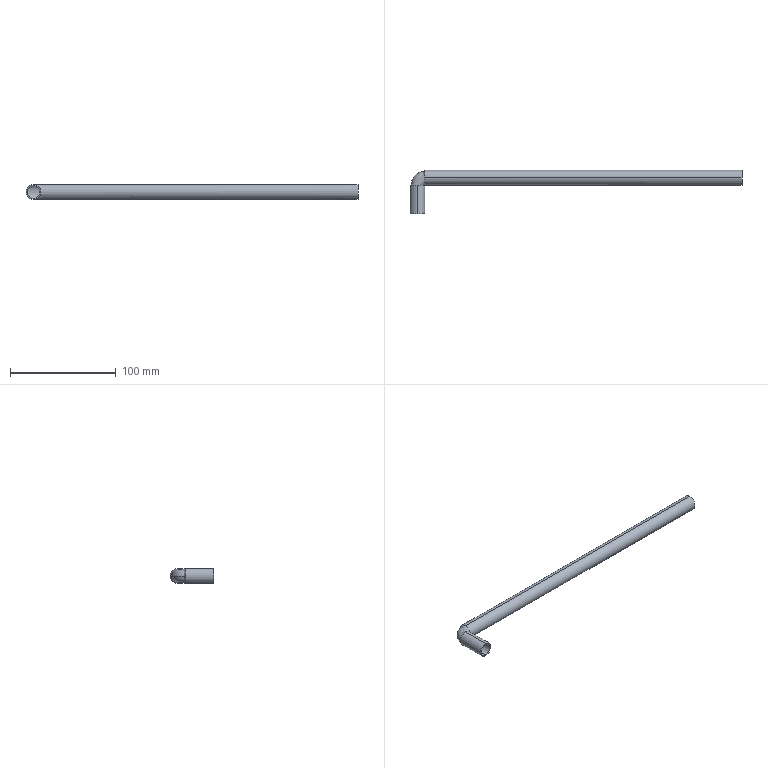Part | NX | features BREP 1 | 1 solid | 13 faces | box 314 x 41 x 14 mm | volume 13804 mm3 | cylinder 8 | torus 3 | plane 2 | commonest cylinder face diameters 12 x4 14 x4
STEP:
#1=CARTESIAN_POINT('',(0.,27.,6.));
#2=VERTEX_POINT('',#1);
#3=CARTESIAN_POINT('',(-6.,27.,0.));
#4=VERTEX_POINT('',#3);
#5=CARTESIAN_POINT('',(0.,27.,0.));
#6=DIRECTION('',(0.,-1.,0.));
#7=DIRECTION('',(0.,0.,1.));
#8=AXIS2_PLACEMENT_3D('',#5,#6,#7);
#9=CIRCLE('',#8,6.);
#10=EDGE_CURVE('',#2,#4,#9,.T.);
#11=ORIENTED_EDGE('',*,*,#10,.T.);
#12=CARTESIAN_POINT('',(7.,40.,0.));
#13=VERTEX_POINT('',#12);
#14=CARTESIAN_POINT('',(7.,27.,0.));
#15=DIRECTION('',(0.,0.,-1.));
#16=DIRECTION('',(0.,1.,0.));
#17=AXIS2_PLACEMENT_3D('',#14,#15,#16);
#18=CIRCLE('',#17,13.);
#19=EDGE_CURVE('',#4,#13,#18,.T.);
#20=ORIENTED_EDGE('',*,*,#19,.T.);
#21=CARTESIAN_POINT('',(7.,34.,6.));
#22=VERTEX_POINT('',#21);
#23=CARTESIAN_POINT('',(7.,34.,0.));
#24=DIRECTION('',(-1.,0.,0.));
#25=DIRECTION('',(0.,0.,1.));
#26=AXIS2_PLACEMENT_3D('',#23,#24,#25);
#27=CIRCLE('',#26,6.);
#28=EDGE_CURVE('',#22,#13,#27,.T.);
#29=ORIENTED_EDGE('',*,*,#28,.F.);
#30=CARTESIAN_POINT('',(7.,28.,0.));
#31=VERTEX_POINT('',#30);
#32=CARTESIAN_POINT('',(7.,34.,0.));
#33=DIRECTION('',(-1.,0.,0.));
#34=DIRECTION('',(0.,0.,1.));
#35=AXIS2_PLACEMENT_3D('',#32,#33,#34);
#36=CIRCLE('',#35,6.);
#37=EDGE_CURVE('',#31,#22,#36,.T.);
#38=ORIENTED_EDGE('',*,*,#37,.F.);
#39=CARTESIAN_POINT('',(6.,27.,0.));
#40=VERTEX_POINT('',#39);
#41=CARTESIAN_POINT('',(7.,27.,0.));
#42=DIRECTION('',(0.,0.,-1.));
#43=DIRECTION('',(0.,1.,0.));
#44=AXIS2_PLACEMENT_3D('',#41,#42,#43);
#45=CIRCLE('',#44,1.);
#46=EDGE_CURVE('',#40,#31,#45,.T.);
#47=ORIENTED_EDGE('',*,*,#46,.F.);
#48=CARTESIAN_POINT('',(0.,27.,0.));
#49=DIRECTION('',(0.,-1.,0.));
#50=DIRECTION('',(0.,0.,1.));
#51=AXIS2_PLACEMENT_3D('',#48,#49,#50);
#52=CIRCLE('',#51,6.);
#53=EDGE_CURVE('',#40,#2,#52,.T.);
#54=ORIENTED_EDGE('',*,*,#53,.T.);
#55=EDGE_LOOP('',(#11,#20,#29,#38,#47,#54));
#56=FACE_BOUND('',#55,.T.);
#57=CARTESIAN_POINT('',(7.,27.,0.));
#58=DIRECTION('',(0.,0.,-1.));
#59=DIRECTION('',(1.,0.,0.));
#60=AXIS2_PLACEMENT_3D('',#57,#58,#59);
#61=TOROIDAL_SURFACE('',#60,7.,6.);
#62=ADVANCED_FACE('',(#56),#61,.F.);
#63=CARTESIAN_POINT('',(7.,34.,-6.));
#64=VERTEX_POINT('',#63);
#65=CARTESIAN_POINT('',(7.,34.,0.));
#66=DIRECTION('',(-1.,0.,0.));
#67=DIRECTION('',(0.,0.,1.));
#68=AXIS2_PLACEMENT_3D('',#65,#66,#67);
#69=CIRCLE('',#68,6.);
#70=EDGE_CURVE('',#64,#31,#69,.T.);
#71=ORIENTED_EDGE('',*,*,#70,.T.);
#72=ORIENTED_EDGE('',*,*,#37,.T.);
#73=CARTESIAN_POINT('',(307.,34.,6.));
#74=VERTEX_POINT('',#73);
#75=CARTESIAN_POINT('',(7.,34.,6.));
#76=DIRECTION('',(1.,0.,0.));
#77=VECTOR('',#76,1000.);
#78=LINE('',#75,#77);
#79=EDGE_CURVE('',#74,#22,#78,.F.);
#80=ORIENTED_EDGE('',*,*,#79,.F.);
#81=CARTESIAN_POINT('',(307.,34.,-6.));
#82=VERTEX_POINT('',#81);
#83=CARTESIAN_POINT('',(307.,34.,0.));
#84=DIRECTION('',(-1.,0.,0.));
#85=DIRECTION('',(0.,0.,1.));
#86=AXIS2_PLACEMENT_3D('',#83,#84,#85);
#87=CIRCLE('',#86,6.);
#88=EDGE_CURVE('',#82,#74,#87,.T.);
#89=ORIENTED_EDGE('',*,*,#88,.F.);
#90=CARTESIAN_POINT('',(7.,34.,-6.));
#91=DIRECTION('',(1.,0.,0.));
#92=VECTOR('',#91,1000.);
#93=LINE('',#90,#92);
#94=EDGE_CURVE('',#82,#64,#93,.F.);
#95=ORIENTED_EDGE('',*,*,#94,.T.);
#96=EDGE_LOOP('',(#71,#72,#80,#89,#95));
#97=FACE_BOUND('',#96,.T.);
#98=CARTESIAN_POINT('',(7.,34.,0.));
#99=DIRECTION('',(1.,0.,0.));
#100=DIRECTION('',(0.,0.,1.));
#101=AXIS2_PLACEMENT_3D('',#98,#99,#100);
#102=CYLINDRICAL_SURFACE('',#101,6.);
#103=ADVANCED_FACE('',(#97),#102,.F.);
#104=CARTESIAN_POINT('',(0.,0.,6.));
#105=VERTEX_POINT('',#104);
#106=CARTESIAN_POINT('',(0.,0.,-6.));
#107=VERTEX_POINT('',#106);
#108=CARTESIAN_POINT('',(0.,0.,0.));
#109=DIRECTION('',(0.,-1.,0.));
#110=DIRECTION('',(0.,0.,1.));
#111=AXIS2_PLACEMENT_3D('',#108,#109,#110);
#112=CIRCLE('',#111,6.);
#113=EDGE_CURVE('',#105,#107,#112,.T.);
#114=ORIENTED_EDGE('',*,*,#113,.T.);
#115=CARTESIAN_POINT('',(0.,27.,-6.));
#116=VERTEX_POINT('',#115);
#117=CARTESIAN_POINT('',(0.,0.,-6.));
#118=DIRECTION('',(0.,1.,0.));
#119=VECTOR('',#118,1000.);
#120=LINE('',#117,#119);
#121=EDGE_CURVE('',#107,#116,#120,.T.);
#122=ORIENTED_EDGE('',*,*,#121,.T.);
#123=CARTESIAN_POINT('',(0.,27.,0.));
#124=DIRECTION('',(0.,-1.,0.));
#125=DIRECTION('',(0.,0.,1.));
#126=AXIS2_PLACEMENT_3D('',#123,#124,#125);
#127=CIRCLE('',#126,6.);
#128=EDGE_CURVE('',#4,#116,#127,.T.);
#129=ORIENTED_EDGE('',*,*,#128,.F.);
#130=ORIENTED_EDGE('',*,*,#10,.F.);
#131=CARTESIAN_POINT('',(0.,0.,6.));
#132=DIRECTION('',(0.,1.,0.));
#133=VECTOR('',#132,1000.);
#134=LINE('',#131,#133);
#135=EDGE_CURVE('',#105,#2,#134,.T.);
#136=ORIENTED_EDGE('',*,*,#135,.F.);
#137=EDGE_LOOP('',(#114,#122,#129,#130,#136));
#138=FACE_BOUND('',#137,.T.);
#139=CARTESIAN_POINT('',(0.,0.,0.));
#140=DIRECTION('',(0.,1.,0.));
#141=DIRECTION('',(0.,0.,-1.));
#142=AXIS2_PLACEMENT_3D('',#139,#140,#141);
#143=CYLINDRICAL_SURFACE('',#142,6.);
#144=ADVANCED_FACE('',(#138),#143,.F.);
#145=CARTESIAN_POINT('',(7.,34.,-7.));
#146=VERTEX_POINT('',#145);
#147=CARTESIAN_POINT('',(7.,34.,7.));
#148=VERTEX_POINT('',#147);
#149=CARTESIAN_POINT('',(7.,34.,0.));
#150=DIRECTION('',(1.,0.,0.));
#151=DIRECTION('',(0.,0.,1.));
#152=AXIS2_PLACEMENT_3D('',#149,#150,#151);
#153=CIRCLE('',#152,7.);
#154=EDGE_CURVE('',#146,#148,#153,.T.);
#155=ORIENTED_EDGE('',*,*,#154,.T.);
#156=CARTESIAN_POINT('',(307.,34.,7.));
#157=VERTEX_POINT('',#156);
#158=CARTESIAN_POINT('',(7.,34.,7.));
#159=DIRECTION('',(1.,0.,0.));
#160=VECTOR('',#159,1000.);
#161=LINE('',#158,#160);
#162=EDGE_CURVE('',#157,#148,#161,.F.);
#163=ORIENTED_EDGE('',*,*,#162,.F.);
#164=CARTESIAN_POINT('',(307.,34.,-7.));
#165=VERTEX_POINT('',#164);
#166=CARTESIAN_POINT('',(307.,34.,0.));
#167=DIRECTION('',(1.,0.,0.));
#168=DIRECTION('',(0.,0.,1.));
#169=AXIS2_PLACEMENT_3D('',#166,#167,#168);
#170=CIRCLE('',#169,7.);
#171=EDGE_CURVE('',#165,#157,#170,.T.);
#172=ORIENTED_EDGE('',*,*,#171,.F.);
#173=CARTESIAN_POINT('',(7.,34.,-7.));
#174=DIRECTION('',(1.,0.,0.));
#175=VECTOR('',#174,1000.);
#176=LINE('',#173,#175);
#177=EDGE_CURVE('',#165,#146,#176,.F.);
#178=ORIENTED_EDGE('',*,*,#177,.T.);
#179=EDGE_LOOP('',(#155,#163,#172,#178));
#180=FACE_BOUND('',#179,.T.);
#181=CARTESIAN_POINT('',(7.,34.,0.));
#182=DIRECTION('',(1.,0.,0.));
#183=DIRECTION('',(0.,0.,1.));
#184=AXIS2_PLACEMENT_3D('',#181,#182,#183);
#185=CYLINDRICAL_SURFACE('',#184,7.);
#186=ADVANCED_FACE('',(#180),#185,.T.);
#187=CARTESIAN_POINT('',(0.,0.,7.));
#188=VERTEX_POINT('',#187);
#189=CARTESIAN_POINT('',(0.,0.,-7.));
#190=VERTEX_POINT('',#189);
#191=CARTESIAN_POINT('',(0.,0.,0.));
#192=DIRECTION('',(0.,1.,0.));
#193=DIRECTION('',(0.,0.,1.));
#194=AXIS2_PLACEMENT_3D('',#191,#192,#193);
#195=CIRCLE('',#194,7.);
#196=EDGE_CURVE('',#188,#190,#195,.T.);
#197=ORIENTED_EDGE('',*,*,#196,.T.);
#198=CARTESIAN_POINT('',(0.,27.,-7.));
#199=VERTEX_POINT('',#198);
#200=CARTESIAN_POINT('',(0.,0.,-7.));
#201=DIRECTION('',(0.,1.,0.));
#202=VECTOR('',#201,1000.);
#203=LINE('',#200,#202);
#204=EDGE_CURVE('',#190,#199,#203,.T.);
#205=ORIENTED_EDGE('',*,*,#204,.T.);
#206=CARTESIAN_POINT('',(7.,27.,0.));
#207=VERTEX_POINT('',#206);
#208=CARTESIAN_POINT('',(0.,27.,0.));
#209=DIRECTION('',(0.,1.,0.));
#210=DIRECTION('',(0.,0.,1.));
#211=AXIS2_PLACEMENT_3D('',#208,#209,#210);
#212=CIRCLE('',#211,7.);
#213=EDGE_CURVE('',#207,#199,#212,.T.);
#214=ORIENTED_EDGE('',*,*,#213,.F.);
#215=CARTESIAN_POINT('',(0.,27.,7.));
#216=VERTEX_POINT('',#215);
#217=CARTESIAN_POINT('',(0.,27.,0.));
#218=DIRECTION('',(0.,1.,0.));
#219=DIRECTION('',(0.,0.,1.));
#220=AXIS2_PLACEMENT_3D('',#217,#218,#219);
#221=CIRCLE('',#220,7.);
#222=EDGE_CURVE('',#216,#207,#221,.T.);
#223=ORIENTED_EDGE('',*,*,#222,.F.);
#224=CARTESIAN_POINT('',(0.,0.,7.));
#225=DIRECTION('',(0.,1.,0.));
#226=VECTOR('',#225,1000.);
#227=LINE('',#224,#226);
#228=EDGE_CURVE('',#188,#216,#227,.T.);
#229=ORIENTED_EDGE('',*,*,#228,.F.);
#230=EDGE_LOOP('',(#197,#205,#214,#223,#229));
#231=FACE_BOUND('',#230,.T.);
#232=CARTESIAN_POINT('',(0.,0.,0.));
#233=DIRECTION('',(0.,1.,0.));
#234=DIRECTION('',(0.,0.,-1.));
#235=AXIS2_PLACEMENT_3D('',#232,#233,#234);
#236=CYLINDRICAL_SURFACE('',#235,7.);
#237=ADVANCED_FACE('',(#231),#236,.T.);
#238=ORIENTED_EDGE('',*,*,#79,.T.);
#239=ORIENTED_EDGE('',*,*,#28,.T.);
#240=CARTESIAN_POINT('',(7.,34.,0.));
#241=DIRECTION('',(-1.,0.,0.));
#242=DIRECTION('',(0.,0.,1.));
#243=AXIS2_PLACEMENT_3D('',#240,#241,#242);
#244=CIRCLE('',#243,6.);
#245=EDGE_CURVE('',#13,#64,#244,.T.);
#246=ORIENTED_EDGE('',*,*,#245,.T.);
#247=ORIENTED_EDGE('',*,*,#94,.F.);
#248=CARTESIAN_POINT('',(307.,34.,0.));
#249=DIRECTION('',(-1.,0.,0.));
#250=DIRECTION('',(0.,0.,1.));
#251=AXIS2_PLACEMENT_3D('',#248,#249,#250);
#252=CIRCLE('',#251,6.);
#253=EDGE_CURVE('',#74,#82,#252,.T.);
#254=ORIENTED_EDGE('',*,*,#253,.F.);
#255=EDGE_LOOP('',(#238,#239,#246,#247,#254));
#256=FACE_BOUND('',#255,.T.);
#257=CARTESIAN_POINT('',(7.,34.,0.));
#258=DIRECTION('',(1.,0.,0.));
#259=DIRECTION('',(0.,0.,1.));
#260=AXIS2_PLACEMENT_3D('',#257,#258,#259);
#261=CYLINDRICAL_SURFACE('',#260,6.);
#262=ADVANCED_FACE('',(#256),#261,.F.);
#263=ORIENTED_EDGE('',*,*,#19,.F.);
#264=ORIENTED_EDGE('',*,*,#128,.T.);
#265=CARTESIAN_POINT('',(0.,27.,0.));
#266=DIRECTION('',(0.,-1.,0.));
#267=DIRECTION('',(0.,0.,1.));
#268=AXIS2_PLACEMENT_3D('',#265,#266,#267);
#269=CIRCLE('',#268,6.);
#270=EDGE_CURVE('',#116,#40,#269,.T.);
#271=ORIENTED_EDGE('',*,*,#270,.T.);
#272=ORIENTED_EDGE('',*,*,#46,.T.);
#273=ORIENTED_EDGE('',*,*,#70,.F.);
#274=ORIENTED_EDGE('',*,*,#245,.F.);
#275=EDGE_LOOP('',(#263,#264,#271,#272,#273,#274));
#276=FACE_BOUND('',#275,.T.);
#277=CARTESIAN_POINT('',(7.,27.,0.));
#278=DIRECTION('',(0.,0.,-1.));
#279=DIRECTION('',(1.,0.,0.));
#280=AXIS2_PLACEMENT_3D('',#277,#278,#279);
#281=TOROIDAL_SURFACE('',#280,7.,6.);
#282=ADVANCED_FACE('',(#276),#281,.F.);
#283=ORIENTED_EDGE('',*,*,#121,.F.);
#284=CARTESIAN_POINT('',(0.,0.,0.));
#285=DIRECTION('',(0.,-1.,0.));
#286=DIRECTION('',(0.,0.,1.));
#287=AXIS2_PLACEMENT_3D('',#284,#285,#286);
#288=CIRCLE('',#287,6.);
#289=EDGE_CURVE('',#107,#105,#288,.T.);
#290=ORIENTED_EDGE('',*,*,#289,.T.);
#291=ORIENTED_EDGE('',*,*,#135,.T.);
#292=ORIENTED_EDGE('',*,*,#53,.F.);
#293=ORIENTED_EDGE('',*,*,#270,.F.);
#294=EDGE_LOOP('',(#283,#290,#291,#292,#293));
#295=FACE_BOUND('',#294,.T.);
#296=CARTESIAN_POINT('',(0.,0.,0.));
#297=DIRECTION('',(0.,1.,0.));
#298=DIRECTION('',(0.,0.,-1.));
#299=AXIS2_PLACEMENT_3D('',#296,#297,#298);
#300=CYLINDRICAL_SURFACE('',#299,6.);
#301=ADVANCED_FACE('',(#295),#300,.F.);
#302=ORIENTED_EDGE('',*,*,#171,.T.);
#303=CARTESIAN_POINT('',(307.,34.,0.));
#304=DIRECTION('',(1.,0.,0.));
#305=DIRECTION('',(0.,0.,1.));
#306=AXIS2_PLACEMENT_3D('',#303,#304,#305);
#307=CIRCLE('',#306,7.);
#308=EDGE_CURVE('',#157,#165,#307,.T.);
#309=ORIENTED_EDGE('',*,*,#308,.T.);
#310=EDGE_LOOP('',(#302,#309));
#311=FACE_BOUND('',#310,.T.);
#312=ORIENTED_EDGE('',*,*,#88,.T.);
#313=ORIENTED_EDGE('',*,*,#253,.T.);
#314=EDGE_LOOP('',(#312,#313));
#315=FACE_BOUND('',#314,.T.);
#316=CARTESIAN_POINT('',(307.,34.,0.));
#317=DIRECTION('',(1.,0.,0.));
#318=DIRECTION('',(0.,1.,0.));
#319=AXIS2_PLACEMENT_3D('',#316,#317,#318);
#320=PLANE('',#319);
#321=ADVANCED_FACE('',(#311,#315),#320,.T.);
#322=ORIENTED_EDGE('',*,*,#196,.F.);
#323=CARTESIAN_POINT('',(0.,0.,0.));
#324=DIRECTION('',(0.,1.,0.));
#325=DIRECTION('',(0.,0.,1.));
#326=AXIS2_PLACEMENT_3D('',#323,#324,#325);
#327=CIRCLE('',#326,7.);
#328=EDGE_CURVE('',#190,#188,#327,.T.);
#329=ORIENTED_EDGE('',*,*,#328,.F.);
#330=EDGE_LOOP('',(#322,#329));
#331=FACE_BOUND('',#330,.T.);
#332=ORIENTED_EDGE('',*,*,#113,.F.);
#333=ORIENTED_EDGE('',*,*,#289,.F.);
#334=EDGE_LOOP('',(#332,#333));
#335=FACE_BOUND('',#334,.T.);
#336=CARTESIAN_POINT('',(0.,0.,0.));
#337=DIRECTION('',(0.,1.,0.));
#338=DIRECTION('',(0.,0.,1.));
#339=AXIS2_PLACEMENT_3D('',#336,#337,#338);
#340=PLANE('',#339);
#341=ADVANCED_FACE('',(#331,#335),#340,.F.);
#342=ORIENTED_EDGE('',*,*,#162,.T.);
#343=CARTESIAN_POINT('',(7.,34.,0.));
#344=DIRECTION('',(1.,0.,0.));
#345=DIRECTION('',(0.,0.,1.));
#346=AXIS2_PLACEMENT_3D('',#343,#344,#345);
#347=CIRCLE('',#346,7.);
#348=EDGE_CURVE('',#148,#207,#347,.T.);
#349=ORIENTED_EDGE('',*,*,#348,.T.);
#350=CARTESIAN_POINT('',(7.,34.,0.));
#351=DIRECTION('',(1.,0.,0.));
#352=DIRECTION('',(0.,0.,1.));
#353=AXIS2_PLACEMENT_3D('',#350,#351,#352);
#354=CIRCLE('',#353,7.);
#355=EDGE_CURVE('',#207,#146,#354,.T.);
#356=ORIENTED_EDGE('',*,*,#355,.T.);
#357=ORIENTED_EDGE('',*,*,#177,.F.);
#358=ORIENTED_EDGE('',*,*,#308,.F.);
#359=EDGE_LOOP('',(#342,#349,#356,#357,#358));
#360=FACE_BOUND('',#359,.T.);
#361=CARTESIAN_POINT('',(7.,34.,0.));
#362=DIRECTION('',(1.,0.,0.));
#363=DIRECTION('',(0.,0.,1.));
#364=AXIS2_PLACEMENT_3D('',#361,#362,#363);
#365=CYLINDRICAL_SURFACE('',#364,7.);
#366=ADVANCED_FACE('',(#360),#365,.T.);
#367=ORIENTED_EDGE('',*,*,#355,.F.);
#368=ORIENTED_EDGE('',*,*,#213,.T.);
#369=CARTESIAN_POINT('',(0.,27.,0.));
#370=DIRECTION('',(0.,1.,0.));
#371=DIRECTION('',(0.,0.,1.));
#372=AXIS2_PLACEMENT_3D('',#369,#370,#371);
#373=CIRCLE('',#372,7.);
#374=EDGE_CURVE('',#199,#216,#373,.T.);
#375=ORIENTED_EDGE('',*,*,#374,.T.);
#376=ORIENTED_EDGE('',*,*,#222,.T.);
#377=ORIENTED_EDGE('',*,*,#348,.F.);
#378=ORIENTED_EDGE('',*,*,#154,.F.);
#379=EDGE_LOOP('',(#367,#368,#375,#376,#377,#378));
#380=FACE_BOUND('',#379,.T.);
#381=CARTESIAN_POINT('',(7.,27.,0.));
#382=DIRECTION('',(0.,0.,-1.));
#383=DIRECTION('',(1.,0.,0.));
#384=AXIS2_PLACEMENT_3D('',#381,#382,#383);
#385=TOROIDAL_SURFACE('',#384,7.,7.);
#386=ADVANCED_FACE('',(#380),#385,.T.);
#387=ORIENTED_EDGE('',*,*,#204,.F.);
#388=ORIENTED_EDGE('',*,*,#328,.T.);
#389=ORIENTED_EDGE('',*,*,#228,.T.);
#390=ORIENTED_EDGE('',*,*,#374,.F.);
#391=EDGE_LOOP('',(#387,#388,#389,#390));
#392=FACE_BOUND('',#391,.T.);
#393=CARTESIAN_POINT('',(0.,0.,0.));
#394=DIRECTION('',(0.,1.,0.));
#395=DIRECTION('',(0.,0.,-1.));
#396=AXIS2_PLACEMENT_3D('',#393,#394,#395);
#397=CYLINDRICAL_SURFACE('',#396,7.);
#398=ADVANCED_FACE('',(#392),#397,.T.);
#399=CLOSED_SHELL('',(#62,#103,#144,#186,#237,#262,#282,#301,#321,#341,#366,#386,#398));
#400=MANIFOLD_SOLID_BREP('',#399);
#401=(LENGTH_UNIT()NAMED_UNIT(*)SI_UNIT(.MILLI.,.METRE.));
#402=UNCERTAINTY_MEASURE_WITH_UNIT(LENGTH_MEASURE(0.00001),#401,'','');
#403=(NAMED_UNIT(*)PLANE_ANGLE_UNIT()SI_UNIT($,.RADIAN.));
#404=(NAMED_UNIT(*)SI_UNIT($,.STERADIAN.)SOLID_ANGLE_UNIT());
#405=(GEOMETRIC_REPRESENTATION_CONTEXT(3)GLOBAL_UNCERTAINTY_ASSIGNED_CONTEXT((#402))GLOBAL_UNIT_ASSIGNED_CONTEXT((#401,#403,#404))REPRESENTATION_CONTEXT('',''));
#406=ADVANCED_BREP_SHAPE_REPRESENTATION('',(#400),#405);